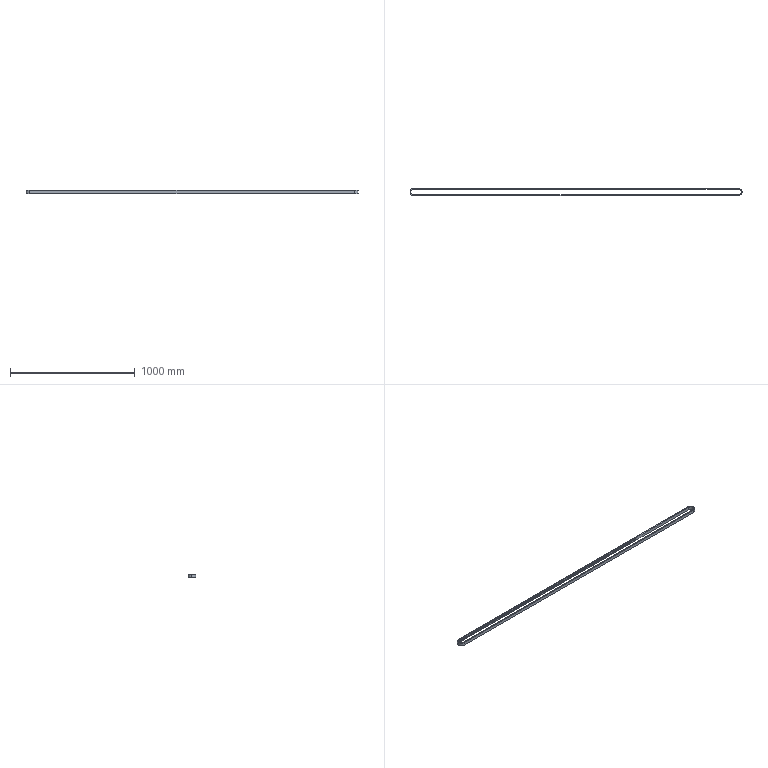Part | SolidWorks | features BaseBody 1 | 1 solid | 812 faces | box 2662 x 62 x 25 mm | volume 852176 mm3 | plane 806 | cylinder 6 | commonest cylinder face diameters 48 x3 62 x3